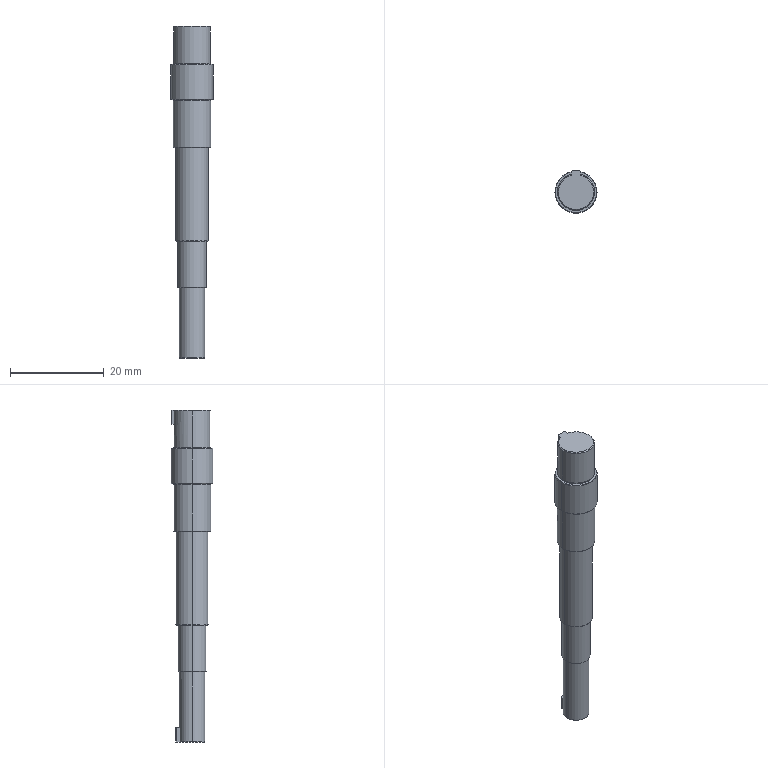Part | SolidWorks | features ICE 9, Chamfer 2, Fillet 2, Extrusion 1 | 1 solid | 53 faces | box 9 x 9 x 71 mm | volume 2813 mm3 | cylinder 20 | plane 17 | cone 16 | commonest cylinder face diameters 0.4 x4 7.8 x4 5.5 x2 6 x2 7 x2 7.9 x2
STEP:
#1=CARTESIAN_POINT('',(-2.65,0.,-63.));
#2=VERTEX_POINT('',#1);
#3=CARTESIAN_POINT('',(-1.,2.454,-63.));
#4=VERTEX_POINT('',#3);
#5=CARTESIAN_POINT('',(0.,0.,-63.));
#6=DIRECTION('',(0.,0.,-1.));
#7=DIRECTION('',(-1.,0.,0.));
#8=AXIS2_PLACEMENT_3D('',#5,#6,#7);
#9=CIRCLE('',#8,2.65);
#10=EDGE_CURVE('',#2,#4,#9,.T.);
#11=ORIENTED_EDGE('',*,*,#10,.F.);
#12=CARTESIAN_POINT('',(-2.75,0.,-62.9));
#13=VERTEX_POINT('',#12);
#14=CARTESIAN_POINT('',(-2.65,0.,-63.));
#15=DIRECTION('',(-0.7071,0.,0.7071));
#16=VECTOR('',#15,1000.);
#17=LINE('',#14,#16);
#18=EDGE_CURVE('',#2,#13,#17,.T.);
#19=ORIENTED_EDGE('',*,*,#18,.T.);
#20=CARTESIAN_POINT('',(-1.,2.562,-62.9));
#21=VERTEX_POINT('',#20);
#22=CARTESIAN_POINT('',(0.,0.,-62.9));
#23=DIRECTION('',(0.,0.,1.));
#24=DIRECTION('',(-1.,0.,0.));
#25=AXIS2_PLACEMENT_3D('',#22,#23,#24);
#26=CIRCLE('',#25,2.75);
#27=EDGE_CURVE('',#21,#13,#26,.T.);
#28=ORIENTED_EDGE('',*,*,#27,.F.);
#29=CARTESIAN_POINT('',(-1.,2.454,-63.));
#30=CARTESIAN_POINT('',(-1.,2.49,-62.967));
#31=CARTESIAN_POINT('',(-1.,2.526,-62.933));
#32=CARTESIAN_POINT('',(-1.,2.562,-62.9));
#33=B_SPLINE_CURVE_WITH_KNOTS('',3,(#29,#30,#31,#32),.UNSPECIFIED.,.F.,.F.,(4,4),(0.,0.0001469),.UNSPECIFIED.);
#34=EDGE_CURVE('',#4,#21,#33,.T.);
#35=ORIENTED_EDGE('',*,*,#34,.F.);
#36=EDGE_LOOP('',(#11,#19,#28,#35));
#37=FACE_OUTER_BOUND('',#36,.T.);
#38=CARTESIAN_POINT('',(0.,0.,-63.));
#39=DIRECTION('',(0.,0.,1.));
#40=DIRECTION('',(1.,0.,0.));
#41=AXIS2_PLACEMENT_3D('',#38,#39,#40);
#42=CONICAL_SURFACE('',#41,2.65,0.7854);
#43=ADVANCED_FACE('',(#37),#42,.T.);
#44=ORIENTED_EDGE('',*,*,#18,.F.);
#45=CARTESIAN_POINT('',(2.65,0.,-63.));
#46=VERTEX_POINT('',#45);
#47=CARTESIAN_POINT('',(0.,0.,-63.));
#48=DIRECTION('',(0.,0.,-1.));
#49=DIRECTION('',(-1.,0.,0.));
#50=AXIS2_PLACEMENT_3D('',#47,#48,#49);
#51=CIRCLE('',#50,2.65);
#52=EDGE_CURVE('',#46,#2,#51,.T.);
#53=ORIENTED_EDGE('',*,*,#52,.F.);
#54=CARTESIAN_POINT('',(2.75,0.,-62.9));
#55=VERTEX_POINT('',#54);
#56=CARTESIAN_POINT('',(2.65,0.,-63.));
#57=DIRECTION('',(0.7071,0.,0.7071));
#58=VECTOR('',#57,1000.);
#59=LINE('',#56,#58);
#60=EDGE_CURVE('',#46,#55,#59,.T.);
#61=ORIENTED_EDGE('',*,*,#60,.T.);
#62=CARTESIAN_POINT('',(0.,0.,-62.9));
#63=DIRECTION('',(0.,0.,1.));
#64=DIRECTION('',(-1.,0.,0.));
#65=AXIS2_PLACEMENT_3D('',#62,#63,#64);
#66=CIRCLE('',#65,2.75);
#67=EDGE_CURVE('',#13,#55,#66,.T.);
#68=ORIENTED_EDGE('',*,*,#67,.F.);
#69=EDGE_LOOP('',(#44,#53,#61,#68));
#70=FACE_OUTER_BOUND('',#69,.T.);
#71=CARTESIAN_POINT('',(0.,0.,-63.));
#72=DIRECTION('',(0.,0.,1.));
#73=DIRECTION('',(1.,0.,0.));
#74=AXIS2_PLACEMENT_3D('',#71,#72,#73);
#75=CONICAL_SURFACE('',#74,2.65,0.7854);
#76=ADVANCED_FACE('',(#70),#75,.T.);
#77=CARTESIAN_POINT('',(-2.9,0.,-48.));
#78=VERTEX_POINT('',#77);
#79=CARTESIAN_POINT('',(2.9,0.,-48.));
#80=VERTEX_POINT('',#79);
#81=CARTESIAN_POINT('',(0.,0.,-48.));
#82=DIRECTION('',(0.,0.,-1.));
#83=DIRECTION('',(-1.,0.,0.));
#84=AXIS2_PLACEMENT_3D('',#81,#82,#83);
#85=CIRCLE('',#84,2.9);
#86=EDGE_CURVE('',#78,#80,#85,.T.);
#87=ORIENTED_EDGE('',*,*,#86,.F.);
#88=CARTESIAN_POINT('',(-3.,0.,-47.9));
#89=VERTEX_POINT('',#88);
#90=CARTESIAN_POINT('',(-2.9,0.,-48.));
#91=DIRECTION('',(-0.7071,0.,0.7071));
#92=VECTOR('',#91,1000.);
#93=LINE('',#90,#92);
#94=EDGE_CURVE('',#78,#89,#93,.T.);
#95=ORIENTED_EDGE('',*,*,#94,.T.);
#96=CARTESIAN_POINT('',(3.,0.,-47.9));
#97=VERTEX_POINT('',#96);
#98=CARTESIAN_POINT('',(0.,0.,-47.9));
#99=DIRECTION('',(0.,0.,1.));
#100=DIRECTION('',(-1.,0.,0.));
#101=AXIS2_PLACEMENT_3D('',#98,#99,#100);
#102=CIRCLE('',#101,3.);
#103=EDGE_CURVE('',#97,#89,#102,.T.);
#104=ORIENTED_EDGE('',*,*,#103,.F.);
#105=CARTESIAN_POINT('',(2.9,0.,-48.));
#106=DIRECTION('',(0.7071,0.,0.7071));
#107=VECTOR('',#106,1000.);
#108=LINE('',#105,#107);
#109=EDGE_CURVE('',#80,#97,#108,.T.);
#110=ORIENTED_EDGE('',*,*,#109,.F.);
#111=EDGE_LOOP('',(#87,#95,#104,#110));
#112=FACE_OUTER_BOUND('',#111,.T.);
#113=CARTESIAN_POINT('',(0.,0.,-48.));
#114=DIRECTION('',(0.,0.,1.));
#115=DIRECTION('',(1.,0.,0.));
#116=AXIS2_PLACEMENT_3D('',#113,#114,#115);
#117=CONICAL_SURFACE('',#116,2.9,0.7854);
#118=ADVANCED_FACE('',(#112),#117,.T.);
#119=CARTESIAN_POINT('',(-3.4,0.,-38.));
#120=VERTEX_POINT('',#119);
#121=CARTESIAN_POINT('',(3.4,0.,-38.));
#122=VERTEX_POINT('',#121);
#123=CARTESIAN_POINT('',(0.,0.,-38.));
#124=DIRECTION('',(0.,0.,-1.));
#125=DIRECTION('',(-1.,0.,0.));
#126=AXIS2_PLACEMENT_3D('',#123,#124,#125);
#127=CIRCLE('',#126,3.4);
#128=EDGE_CURVE('',#120,#122,#127,.T.);
#129=ORIENTED_EDGE('',*,*,#128,.F.);
#130=CARTESIAN_POINT('',(-3.5,0.,-37.9));
#131=VERTEX_POINT('',#130);
#132=CARTESIAN_POINT('',(-3.4,0.,-38.));
#133=DIRECTION('',(-0.7071,0.,0.7071));
#134=VECTOR('',#133,1000.);
#135=LINE('',#132,#134);
#136=EDGE_CURVE('',#120,#131,#135,.T.);
#137=ORIENTED_EDGE('',*,*,#136,.T.);
#138=CARTESIAN_POINT('',(3.5,0.,-37.9));
#139=VERTEX_POINT('',#138);
#140=CARTESIAN_POINT('',(0.,0.,-37.9));
#141=DIRECTION('',(0.,0.,1.));
#142=DIRECTION('',(-1.,0.,0.));
#143=AXIS2_PLACEMENT_3D('',#140,#141,#142);
#144=CIRCLE('',#143,3.5);
#145=EDGE_CURVE('',#139,#131,#144,.T.);
#146=ORIENTED_EDGE('',*,*,#145,.F.);
#147=CARTESIAN_POINT('',(3.4,0.,-38.));
#148=DIRECTION('',(0.7071,0.,0.7071));
#149=VECTOR('',#148,1000.);
#150=LINE('',#147,#149);
#151=EDGE_CURVE('',#122,#139,#150,.T.);
#152=ORIENTED_EDGE('',*,*,#151,.F.);
#153=EDGE_LOOP('',(#129,#137,#146,#152));
#154=FACE_OUTER_BOUND('',#153,.T.);
#155=CARTESIAN_POINT('',(0.,0.,-38.));
#156=DIRECTION('',(0.,0.,1.));
#157=DIRECTION('',(1.,0.,0.));
#158=AXIS2_PLACEMENT_3D('',#155,#156,#157);
#159=CONICAL_SURFACE('',#158,3.4,0.7854);
#160=ADVANCED_FACE('',(#154),#159,.T.);
#161=CARTESIAN_POINT('',(-3.9,0.,-18.));
#162=VERTEX_POINT('',#161);
#163=CARTESIAN_POINT('',(3.9,0.,-18.));
#164=VERTEX_POINT('',#163);
#165=CARTESIAN_POINT('',(0.,0.,-18.));
#166=DIRECTION('',(0.,0.,-1.));
#167=DIRECTION('',(-1.,0.,0.));
#168=AXIS2_PLACEMENT_3D('',#165,#166,#167);
#169=CIRCLE('',#168,3.9);
#170=EDGE_CURVE('',#162,#164,#169,.T.);
#171=ORIENTED_EDGE('',*,*,#170,.F.);
#172=CARTESIAN_POINT('',(-4.,0.,-17.9));
#173=VERTEX_POINT('',#172);
#174=CARTESIAN_POINT('',(-3.9,0.,-18.));
#175=DIRECTION('',(-0.7071,0.,0.7071));
#176=VECTOR('',#175,1000.);
#177=LINE('',#174,#176);
#178=EDGE_CURVE('',#162,#173,#177,.T.);
#179=ORIENTED_EDGE('',*,*,#178,.T.);
#180=CARTESIAN_POINT('',(4.,0.,-17.9));
#181=VERTEX_POINT('',#180);
#182=CARTESIAN_POINT('',(0.,0.,-17.9));
#183=DIRECTION('',(0.,0.,1.));
#184=DIRECTION('',(-1.,0.,0.));
#185=AXIS2_PLACEMENT_3D('',#182,#183,#184);
#186=CIRCLE('',#185,4.);
#187=EDGE_CURVE('',#181,#173,#186,.T.);
#188=ORIENTED_EDGE('',*,*,#187,.F.);
#189=CARTESIAN_POINT('',(3.9,0.,-18.));
#190=DIRECTION('',(0.7071,0.,0.7071));
#191=VECTOR('',#190,1000.);
#192=LINE('',#189,#191);
#193=EDGE_CURVE('',#164,#181,#192,.T.);
#194=ORIENTED_EDGE('',*,*,#193,.F.);
#195=EDGE_LOOP('',(#171,#179,#188,#194));
#196=FACE_OUTER_BOUND('',#195,.T.);
#197=CARTESIAN_POINT('',(0.,0.,-18.));
#198=DIRECTION('',(0.,0.,1.));
#199=DIRECTION('',(1.,0.,0.));
#200=AXIS2_PLACEMENT_3D('',#197,#198,#199);
#201=CONICAL_SURFACE('',#200,3.9,0.7854);
#202=ADVANCED_FACE('',(#196),#201,.T.);
#203=CARTESIAN_POINT('',(-4.4,0.,-7.8));
#204=VERTEX_POINT('',#203);
#205=CARTESIAN_POINT('',(4.4,0.,-7.8));
#206=VERTEX_POINT('',#205);
#207=CARTESIAN_POINT('',(0.,0.,-7.8));
#208=DIRECTION('',(0.,0.,-1.));
#209=DIRECTION('',(-1.,0.,0.));
#210=AXIS2_PLACEMENT_3D('',#207,#208,#209);
#211=CIRCLE('',#210,4.4);
#212=EDGE_CURVE('',#204,#206,#211,.T.);
#213=ORIENTED_EDGE('',*,*,#212,.F.);
#214=CARTESIAN_POINT('',(-4.5,0.,-7.7));
#215=VERTEX_POINT('',#214);
#216=CARTESIAN_POINT('',(-4.4,0.,-7.8));
#217=DIRECTION('',(-0.7071,0.,0.7071));
#218=VECTOR('',#217,1000.);
#219=LINE('',#216,#218);
#220=EDGE_CURVE('',#204,#215,#219,.T.);
#221=ORIENTED_EDGE('',*,*,#220,.T.);
#222=CARTESIAN_POINT('',(4.5,0.,-7.7));
#223=VERTEX_POINT('',#222);
#224=CARTESIAN_POINT('',(0.,0.,-7.7));
#225=DIRECTION('',(0.,0.,1.));
#226=DIRECTION('',(-1.,0.,0.));
#227=AXIS2_PLACEMENT_3D('',#224,#225,#226);
#228=CIRCLE('',#227,4.5);
#229=EDGE_CURVE('',#223,#215,#228,.T.);
#230=ORIENTED_EDGE('',*,*,#229,.F.);
#231=CARTESIAN_POINT('',(4.4,0.,-7.8));
#232=DIRECTION('',(0.7071,0.,0.7071));
#233=VECTOR('',#232,1000.);
#234=LINE('',#231,#233);
#235=EDGE_CURVE('',#206,#223,#234,.T.);
#236=ORIENTED_EDGE('',*,*,#235,.F.);
#237=EDGE_LOOP('',(#213,#221,#230,#236));
#238=FACE_OUTER_BOUND('',#237,.T.);
#239=CARTESIAN_POINT('',(0.,0.,-7.8));
#240=DIRECTION('',(0.,0.,1.));
#241=DIRECTION('',(1.,0.,0.));
#242=AXIS2_PLACEMENT_3D('',#239,#240,#241);
#243=CONICAL_SURFACE('',#242,4.4,0.7854);
#244=ADVANCED_FACE('',(#238),#243,.T.);
#245=CARTESIAN_POINT('',(4.4,0.,-0.2));
#246=VERTEX_POINT('',#245);
#247=CARTESIAN_POINT('',(-4.4,0.,-0.2));
#248=VERTEX_POINT('',#247);
#249=CARTESIAN_POINT('',(0.,0.,-0.2));
#250=DIRECTION('',(0.,0.,1.));
#251=DIRECTION('',(-1.,0.,0.));
#252=AXIS2_PLACEMENT_3D('',#249,#250,#251);
#253=CIRCLE('',#252,4.4);
#254=EDGE_CURVE('',#246,#248,#253,.T.);
#255=ORIENTED_EDGE('',*,*,#254,.F.);
#256=CARTESIAN_POINT('',(4.5,0.,-0.3));
#257=VERTEX_POINT('',#256);
#258=CARTESIAN_POINT('',(4.5,0.,-0.3));
#259=DIRECTION('',(0.7071,0.,-0.7071));
#260=VECTOR('',#259,1000.);
#261=LINE('',#258,#260);
#262=EDGE_CURVE('',#246,#257,#261,.T.);
#263=ORIENTED_EDGE('',*,*,#262,.T.);
#264=CARTESIAN_POINT('',(-4.5,0.,-0.3));
#265=VERTEX_POINT('',#264);
#266=CARTESIAN_POINT('',(0.,0.,-0.3));
#267=DIRECTION('',(0.,0.,-1.));
#268=DIRECTION('',(-1.,0.,0.));
#269=AXIS2_PLACEMENT_3D('',#266,#267,#268);
#270=CIRCLE('',#269,4.5);
#271=EDGE_CURVE('',#265,#257,#270,.T.);
#272=ORIENTED_EDGE('',*,*,#271,.F.);
#273=CARTESIAN_POINT('',(-4.5,0.,-0.3));
#274=DIRECTION('',(-0.7071,0.,-0.7071));
#275=VECTOR('',#274,1000.);
#276=LINE('',#273,#275);
#277=EDGE_CURVE('',#248,#265,#276,.T.);
#278=ORIENTED_EDGE('',*,*,#277,.F.);
#279=EDGE_LOOP('',(#255,#263,#272,#278));
#280=FACE_OUTER_BOUND('',#279,.T.);
#281=CARTESIAN_POINT('',(0.,0.,-0.3));
#282=DIRECTION('',(0.,0.,-1.));
#283=DIRECTION('',(-1.,0.,0.));
#284=AXIS2_PLACEMENT_3D('',#281,#282,#283);
#285=CONICAL_SURFACE('',#284,4.5,0.7854);
#286=ADVANCED_FACE('',(#280),#285,.T.);
#287=ORIENTED_EDGE('',*,*,#27,.T.);
#288=CARTESIAN_POINT('',(-2.75,0.,-48.));
#289=VERTEX_POINT('',#288);
#290=CARTESIAN_POINT('',(-2.75,0.,-63.));
#291=DIRECTION('',(0.,0.,1.));
#292=VECTOR('',#291,1000.);
#293=LINE('',#290,#292);
#294=EDGE_CURVE('',#13,#289,#293,.T.);
#295=ORIENTED_EDGE('',*,*,#294,.T.);
#296=CARTESIAN_POINT('',(2.75,0.,-48.));
#297=VERTEX_POINT('',#296);
#298=CARTESIAN_POINT('',(0.,0.,-48.));
#299=DIRECTION('',(0.,0.,-1.));
#300=DIRECTION('',(-1.,0.,0.));
#301=AXIS2_PLACEMENT_3D('',#298,#299,#300);
#302=CIRCLE('',#301,2.75);
#303=EDGE_CURVE('',#289,#297,#302,.T.);
#304=ORIENTED_EDGE('',*,*,#303,.T.);
#305=CARTESIAN_POINT('',(2.75,0.,-63.));
#306=DIRECTION('',(0.,0.,1.));
#307=VECTOR('',#306,1000.);
#308=LINE('',#305,#307);
#309=EDGE_CURVE('',#55,#297,#308,.T.);
#310=ORIENTED_EDGE('',*,*,#309,.F.);
#311=CARTESIAN_POINT('',(1.,2.562,-62.9));
#312=VERTEX_POINT('',#311);
#313=CARTESIAN_POINT('',(0.,0.,-62.9));
#314=DIRECTION('',(0.,0.,1.));
#315=DIRECTION('',(-1.,0.,0.));
#316=AXIS2_PLACEMENT_3D('',#313,#314,#315);
#317=CIRCLE('',#316,2.75);
#318=EDGE_CURVE('',#55,#312,#317,.T.);
#319=ORIENTED_EDGE('',*,*,#318,.T.);
#320=CARTESIAN_POINT('',(1.,2.562,-60.));
#321=VERTEX_POINT('',#320);
#322=CARTESIAN_POINT('',(1.,2.562,-65.209));
#323=DIRECTION('',(0.,0.,1.));
#324=VECTOR('',#323,1000.);
#325=LINE('',#322,#324);
#326=EDGE_CURVE('',#312,#321,#325,.T.);
#327=ORIENTED_EDGE('',*,*,#326,.T.);
#328=CARTESIAN_POINT('',(-1.,2.562,-60.));
#329=VERTEX_POINT('',#328);
#330=CARTESIAN_POINT('',(0.,0.,-60.));
#331=DIRECTION('',(0.,0.,-1.));
#332=DIRECTION('',(-1.,0.,0.));
#333=AXIS2_PLACEMENT_3D('',#330,#331,#332);
#334=CIRCLE('',#333,2.75);
#335=EDGE_CURVE('',#329,#321,#334,.T.);
#336=ORIENTED_EDGE('',*,*,#335,.F.);
#337=CARTESIAN_POINT('',(-1.,2.562,-65.209));
#338=DIRECTION('',(0.,0.,1.));
#339=VECTOR('',#338,1000.);
#340=LINE('',#337,#339);
#341=EDGE_CURVE('',#21,#329,#340,.T.);
#342=ORIENTED_EDGE('',*,*,#341,.F.);
#343=EDGE_LOOP('',(#287,#295,#304,#310,#319,#327,#336,#342));
#344=FACE_OUTER_BOUND('',#343,.T.);
#345=CARTESIAN_POINT('',(0.,0.,-63.));
#346=DIRECTION('',(0.,0.,1.));
#347=DIRECTION('',(1.,0.,0.));
#348=AXIS2_PLACEMENT_3D('',#345,#346,#347);
#349=CYLINDRICAL_SURFACE('',#348,2.75);
#350=ADVANCED_FACE('',(#344),#349,.T.);
#351=ORIENTED_EDGE('',*,*,#103,.T.);
#352=CARTESIAN_POINT('',(-3.,0.,-38.));
#353=VERTEX_POINT('',#352);
#354=CARTESIAN_POINT('',(-3.,0.,-48.));
#355=DIRECTION('',(0.,0.,1.));
#356=VECTOR('',#355,1000.);
#357=LINE('',#354,#356);
#358=EDGE_CURVE('',#89,#353,#357,.T.);
#359=ORIENTED_EDGE('',*,*,#358,.T.);
#360=CARTESIAN_POINT('',(3.,0.,-38.));
#361=VERTEX_POINT('',#360);
#362=CARTESIAN_POINT('',(0.,0.,-38.));
#363=DIRECTION('',(0.,0.,-1.));
#364=DIRECTION('',(-1.,0.,0.));
#365=AXIS2_PLACEMENT_3D('',#362,#363,#364);
#366=CIRCLE('',#365,3.);
#367=EDGE_CURVE('',#353,#361,#366,.T.);
#368=ORIENTED_EDGE('',*,*,#367,.T.);
#369=CARTESIAN_POINT('',(3.,0.,-48.));
#370=DIRECTION('',(0.,0.,1.));
#371=VECTOR('',#370,1000.);
#372=LINE('',#369,#371);
#373=EDGE_CURVE('',#97,#361,#372,.T.);
#374=ORIENTED_EDGE('',*,*,#373,.F.);
#375=EDGE_LOOP('',(#351,#359,#368,#374));
#376=FACE_OUTER_BOUND('',#375,.T.);
#377=CARTESIAN_POINT('',(0.,0.,-48.));
#378=DIRECTION('',(0.,0.,1.));
#379=DIRECTION('',(1.,0.,0.));
#380=AXIS2_PLACEMENT_3D('',#377,#378,#379);
#381=CYLINDRICAL_SURFACE('',#380,3.);
#382=ADVANCED_FACE('',(#376),#381,.T.);
#383=ORIENTED_EDGE('',*,*,#145,.T.);
#384=CARTESIAN_POINT('',(-3.5,0.,-18.));
#385=VERTEX_POINT('',#384);
#386=CARTESIAN_POINT('',(-3.5,0.,-38.));
#387=DIRECTION('',(0.,0.,1.));
#388=VECTOR('',#387,1000.);
#389=LINE('',#386,#388);
#390=EDGE_CURVE('',#131,#385,#389,.T.);
#391=ORIENTED_EDGE('',*,*,#390,.T.);
#392=CARTESIAN_POINT('',(3.5,0.,-18.));
#393=VERTEX_POINT('',#392);
#394=CARTESIAN_POINT('',(0.,0.,-18.));
#395=DIRECTION('',(0.,0.,-1.));
#396=DIRECTION('',(-1.,0.,0.));
#397=AXIS2_PLACEMENT_3D('',#394,#395,#396);
#398=CIRCLE('',#397,3.5);
#399=EDGE_CURVE('',#385,#393,#398,.T.);
#400=ORIENTED_EDGE('',*,*,#399,.T.);
#401=CARTESIAN_POINT('',(3.5,0.,-38.));
#402=DIRECTION('',(0.,0.,1.));
#403=VECTOR('',#402,1000.);
#404=LINE('',#401,#403);
#405=EDGE_CURVE('',#139,#393,#404,.T.);
#406=ORIENTED_EDGE('',*,*,#405,.F.);
#407=EDGE_LOOP('',(#383,#391,#400,#406));
#408=FACE_OUTER_BOUND('',#407,.T.);
#409=CARTESIAN_POINT('',(0.,0.,-38.));
#410=DIRECTION('',(0.,0.,1.));
#411=DIRECTION('',(1.,0.,0.));
#412=AXIS2_PLACEMENT_3D('',#409,#410,#411);
#413=CYLINDRICAL_SURFACE('',#412,3.5);
#414=ADVANCED_FACE('',(#408),#413,.T.);
#415=ORIENTED_EDGE('',*,*,#187,.T.);
#416=CARTESIAN_POINT('',(-4.,0.,-8.));
#417=VERTEX_POINT('',#416);
#418=CARTESIAN_POINT('',(-4.,0.,-18.));
#419=DIRECTION('',(0.,0.,1.));
#420=VECTOR('',#419,1000.);
#421=LINE('',#418,#420);
#422=EDGE_CURVE('',#173,#417,#421,.T.);
#423=ORIENTED_EDGE('',*,*,#422,.T.);
#424=CARTESIAN_POINT('',(4.,0.,-8.));
#425=VERTEX_POINT('',#424);
#426=CARTESIAN_POINT('',(0.,0.,-8.));
#427=DIRECTION('',(0.,0.,-1.));
#428=DIRECTION('',(-1.,0.,0.));
#429=AXIS2_PLACEMENT_3D('',#426,#427,#428);
#430=CIRCLE('',#429,4.);
#431=EDGE_CURVE('',#417,#425,#430,.T.);
#432=ORIENTED_EDGE('',*,*,#431,.T.);
#433=CARTESIAN_POINT('',(4.,0.,-18.));
#434=DIRECTION('',(0.,0.,1.));
#435=VECTOR('',#434,1000.);
#436=LINE('',#433,#435);
#437=EDGE_CURVE('',#181,#425,#436,.T.);
#438=ORIENTED_EDGE('',*,*,#437,.F.);
#439=EDGE_LOOP('',(#415,#423,#432,#438));
#440=FACE_OUTER_BOUND('',#439,.T.);
#441=CARTESIAN_POINT('',(0.,0.,-18.));
#442=DIRECTION('',(0.,0.,1.));
#443=DIRECTION('',(1.,0.,0.));
#444=AXIS2_PLACEMENT_3D('',#441,#442,#443);
#445=CYLINDRICAL_SURFACE('',#444,4.);
#446=ADVANCED_FACE('',(#440),#445,.T.);
#447=CARTESIAN_POINT('',(3.75,0.,8.));
#448=VERTEX_POINT('',#447);
#449=CARTESIAN_POINT('',(1.,3.614,8.));
#450=VERTEX_POINT('',#449);
#451=CARTESIAN_POINT('',(0.,0.,8.));
#452=DIRECTION('',(0.,0.,1.));
#453=DIRECTION('',(1.,0.,0.));
#454=AXIS2_PLACEMENT_3D('',#451,#452,#453);
#455=CIRCLE('',#454,3.75);
#456=EDGE_CURVE('',#448,#450,#455,.T.);
#457=ORIENTED_EDGE('',*,*,#456,.F.);
#458=CARTESIAN_POINT('',(3.95,0.,7.8));
#459=VERTEX_POINT('',#458);
#460=CARTESIAN_POINT('',(3.75,0.,8.));
#461=DIRECTION('',(0.7071,0.,-0.7071));
#462=VECTOR('',#461,1000.);
#463=LINE('',#460,#462);
#464=EDGE_CURVE('',#448,#459,#463,.T.);
#465=ORIENTED_EDGE('',*,*,#464,.T.);
#466=CARTESIAN_POINT('',(1.,3.821,7.8));
#467=VERTEX_POINT('',#466);
#468=CARTESIAN_POINT('',(0.,0.,7.8));
#469=DIRECTION('',(0.,0.,-1.));
#470=DIRECTION('',(1.,0.,0.));
#471=AXIS2_PLACEMENT_3D('',#468,#469,#470);
#472=CIRCLE('',#471,3.95);
#473=EDGE_CURVE('',#467,#459,#472,.T.);
#474=ORIENTED_EDGE('',*,*,#473,.F.);
#475=CARTESIAN_POINT('',(1.,3.614,8.));
#476=CARTESIAN_POINT('',(1.,3.683,7.933));
#477=CARTESIAN_POINT('',(1.,3.752,7.867));
#478=CARTESIAN_POINT('',(1.,3.821,7.8));
#479=B_SPLINE_CURVE_WITH_KNOTS('',3,(#475,#476,#477,#478),.UNSPECIFIED.,.F.,.F.,(4,4),(0.,0.0002879),.UNSPECIFIED.);
#480=EDGE_CURVE('',#450,#467,#479,.T.);
#481=ORIENTED_EDGE('',*,*,#480,.F.);
#482=EDGE_LOOP('',(#457,#465,#474,#481));
#483=FACE_OUTER_BOUND('',#482,.T.);
#484=CARTESIAN_POINT('',(0.,0.,8.));
#485=DIRECTION('',(0.,0.,-1.));
#486=DIRECTION('',(-1.,0.,0.));
#487=AXIS2_PLACEMENT_3D('',#484,#485,#486);
#488=CONICAL_SURFACE('',#487,3.75,0.7854);
#489=ADVANCED_FACE('',(#483),#488,.T.);
#490=ORIENTED_EDGE('',*,*,#464,.F.);
#491=CARTESIAN_POINT('',(-3.75,0.,8.));
#492=VERTEX_POINT('',#491);
#493=CARTESIAN_POINT('',(0.,0.,8.));
#494=DIRECTION('',(0.,0.,1.));
#495=DIRECTION('',(1.,0.,0.));
#496=AXIS2_PLACEMENT_3D('',#493,#494,#495);
#497=CIRCLE('',#496,3.75);
#498=EDGE_CURVE('',#492,#448,#497,.T.);
#499=ORIENTED_EDGE('',*,*,#498,.F.);
#500=CARTESIAN_POINT('',(-3.95,0.,7.8));
#501=VERTEX_POINT('',#500);
#502=CARTESIAN_POINT('',(-3.75,0.,8.));
#503=DIRECTION('',(-0.7071,0.,-0.7071));
#504=VECTOR('',#503,1000.);
#505=LINE('',#502,#504);
#506=EDGE_CURVE('',#492,#501,#505,.T.);
#507=ORIENTED_EDGE('',*,*,#506,.T.);
#508=CARTESIAN_POINT('',(0.,0.,7.8));
#509=DIRECTION('',(0.,0.,-1.));
#510=DIRECTION('',(1.,0.,0.));
#511=AXIS2_PLACEMENT_3D('',#508,#509,#510);
#512=CIRCLE('',#511,3.95);
#513=EDGE_CURVE('',#459,#501,#512,.T.);
#514=ORIENTED_EDGE('',*,*,#513,.F.);
#515=EDGE_LOOP('',(#490,#499,#507,#514));
#516=FACE_OUTER_BOUND('',#515,.T.);
#517=CARTESIAN_POINT('',(0.,0.,8.));
#518=DIRECTION('',(0.,0.,-1.));
#519=DIRECTION('',(-1.,0.,0.));
#520=AXIS2_PLACEMENT_3D('',#517,#518,#519);
#521=CONICAL_SURFACE('',#520,3.75,0.7854);
#522=ADVANCED_FACE('',(#516),#521,.T.);
#523=CARTESIAN_POINT('',(-3.9,0.,-8.));
#524=VERTEX_POINT('',#523);
#525=CARTESIAN_POINT('',(3.9,0.,-8.));
#526=VERTEX_POINT('',#525);
#527=CARTESIAN_POINT('',(0.,0.,-8.));
#528=DIRECTION('',(0.,0.,-1.));
#529=DIRECTION('',(-1.,0.,0.));
#530=AXIS2_PLACEMENT_3D('',#527,#528,#529);
#531=CIRCLE('',#530,3.9);
#532=EDGE_CURVE('',#524,#526,#531,.T.);
#533=ORIENTED_EDGE('',*,*,#532,.F.);
#534=CARTESIAN_POINT('',(-3.9,0.,-7.8));
#535=VERTEX_POINT('',#534);
#536=CARTESIAN_POINT('',(-3.9,0.,-8.));
#537=DIRECTION('',(0.,0.,1.));
#538=VECTOR('',#537,1000.);
#539=LINE('',#536,#538);
#540=EDGE_CURVE('',#524,#535,#539,.T.);
#541=ORIENTED_EDGE('',*,*,#540,.T.);
#542=CARTESIAN_POINT('',(3.9,0.,-7.8));
#543=VERTEX_POINT('',#542);
#544=CARTESIAN_POINT('',(0.,0.,-7.8));
#545=DIRECTION('',(0.,0.,-1.));
#546=DIRECTION('',(-1.,0.,0.));
#547=AXIS2_PLACEMENT_3D('',#544,#545,#546);
#548=CIRCLE('',#547,3.9);
#549=EDGE_CURVE('',#535,#543,#548,.T.);
#550=ORIENTED_EDGE('',*,*,#549,.T.);
#551=CARTESIAN_POINT('',(3.9,0.,-8.));
#552=DIRECTION('',(0.,0.,1.));
#553=VECTOR('',#552,1000.);
#554=LINE('',#551,#553);
#555=EDGE_CURVE('',#526,#543,#554,.T.);
#556=ORIENTED_EDGE('',*,*,#555,.F.);
#557=EDGE_LOOP('',(#533,#541,#550,#556));
#558=FACE_OUTER_BOUND('',#557,.T.);
#559=CARTESIAN_POINT('',(0.,0.,-8.));
#560=DIRECTION('',(0.,0.,1.));
#561=DIRECTION('',(1.,0.,0.));
#562=AXIS2_PLACEMENT_3D('',#559,#560,#561);
#563=CYLINDRICAL_SURFACE('',#562,3.9);
#564=ADVANCED_FACE('',(#558),#563,.T.);
#565=ORIENTED_EDGE('',*,*,#229,.T.);
#566=CARTESIAN_POINT('',(-4.5,0.,-7.8));
#567=DIRECTION('',(0.,0.,1.));
#568=VECTOR('',#567,1000.);
#569=LINE('',#566,#568);
#570=EDGE_CURVE('',#215,#265,#569,.T.);
#571=ORIENTED_EDGE('',*,*,#570,.T.);
#572=ORIENTED_EDGE('',*,*,#271,.T.);
#573=CARTESIAN_POINT('',(4.5,0.,-7.8));
#574=DIRECTION('',(0.,0.,1.));
#575=VECTOR('',#574,1000.);
#576=LINE('',#573,#575);
#577=EDGE_CURVE('',#223,#257,#576,.T.);
#578=ORIENTED_EDGE('',*,*,#577,.F.);
#579=EDGE_LOOP('',(#565,#571,#572,#578));
#580=FACE_OUTER_BOUND('',#579,.T.);
#581=CARTESIAN_POINT('',(0.,0.,-7.8));
#582=DIRECTION('',(0.,0.,1.));
#583=DIRECTION('',(1.,0.,0.));
#584=AXIS2_PLACEMENT_3D('',#581,#582,#583);
#585=CYLINDRICAL_SURFACE('',#584,4.5);
#586=ADVANCED_FACE('',(#580),#585,.T.);
#587=CARTESIAN_POINT('',(-3.9,0.,-0.2));
#588=VERTEX_POINT('',#587);
#589=CARTESIAN_POINT('',(3.9,0.,-0.2));
#590=VERTEX_POINT('',#589);
#591=CARTESIAN_POINT('',(0.,0.,-0.2));
#592=DIRECTION('',(0.,0.,-1.));
#593=DIRECTION('',(-1.,0.,0.));
#594=AXIS2_PLACEMENT_3D('',#591,#592,#593);
#595=CIRCLE('',#594,3.9);
#596=EDGE_CURVE('',#588,#590,#595,.T.);
#597=ORIENTED_EDGE('',*,*,#596,.F.);
#598=CARTESIAN_POINT('',(-3.9,0.,0.));
#599=VERTEX_POINT('',#598);
#600=CARTESIAN_POINT('',(-3.9,0.,-0.2));
#601=DIRECTION('',(0.,0.,1.));
#602=VECTOR('',#601,1000.);
#603=LINE('',#600,#602);
#604=EDGE_CURVE('',#588,#599,#603,.T.);
#605=ORIENTED_EDGE('',*,*,#604,.T.);
#606=CARTESIAN_POINT('',(3.9,0.,0.));
#607=VERTEX_POINT('',#606);
#608=CARTESIAN_POINT('',(0.,0.,0.));
#609=DIRECTION('',(0.,0.,-1.));
#610=DIRECTION('',(-1.,0.,0.));
#611=AXIS2_PLACEMENT_3D('',#608,#609,#610);
#612=CIRCLE('',#611,3.9);
#613=EDGE_CURVE('',#599,#607,#612,.T.);
#614=ORIENTED_EDGE('',*,*,#613,.T.);
#615=CARTESIAN_POINT('',(3.9,0.,-0.2));
#616=DIRECTION('',(0.,0.,1.));
#617=VECTOR('',#616,1000.);
#618=LINE('',#615,#617);
#619=EDGE_CURVE('',#590,#607,#618,.T.);
#620=ORIENTED_EDGE('',*,*,#619,.F.);
#621=EDGE_LOOP('',(#597,#605,#614,#620));
#622=FACE_OUTER_BOUND('',#621,.T.);
#623=CARTESIAN_POINT('',(0.,0.,-0.2));
#624=DIRECTION('',(0.,0.,1.));
#625=DIRECTION('',(1.,0.,0.));
#626=AXIS2_PLACEMENT_3D('',#623,#624,#625);
#627=CYLINDRICAL_SURFACE('',#626,3.9);
#628=ADVANCED_FACE('',(#622),#627,.T.);
#629=ORIENTED_EDGE('',*,*,#473,.T.);
#630=CARTESIAN_POINT('',(3.95,0.,0.));
#631=VERTEX_POINT('',#630);
#632=CARTESIAN_POINT('',(3.95,0.,8.));
#633=DIRECTION('',(0.,0.,-1.));
#634=VECTOR('',#633,1000.);
#635=LINE('',#632,#634);
#636=EDGE_CURVE('',#459,#631,#635,.T.);
#637=ORIENTED_EDGE('',*,*,#636,.T.);
#638=CARTESIAN_POINT('',(-3.95,0.,0.));
#639=VERTEX_POINT('',#638);
#640=CARTESIAN_POINT('',(0.,0.,0.));
#641=DIRECTION('',(0.,0.,1.));
#642=DIRECTION('',(1.,0.,0.));
#643=AXIS2_PLACEMENT_3D('',#640,#641,#642);
#644=CIRCLE('',#643,3.95);
#645=EDGE_CURVE('',#631,#639,#644,.T.);
#646=ORIENTED_EDGE('',*,*,#645,.T.);
#647=CARTESIAN_POINT('',(-3.95,0.,8.));
#648=DIRECTION('',(0.,0.,-1.));
#649=VECTOR('',#648,1000.);
#650=LINE('',#647,#649);
#651=EDGE_CURVE('',#501,#639,#650,.T.);
#652=ORIENTED_EDGE('',*,*,#651,.F.);
#653=CARTESIAN_POINT('',(-1.,3.821,7.8));
#654=VERTEX_POINT('',#653);
#655=CARTESIAN_POINT('',(0.,0.,7.8));
#656=DIRECTION('',(0.,0.,-1.));
#657=DIRECTION('',(1.,0.,0.));
#658=AXIS2_PLACEMENT_3D('',#655,#656,#657);
#659=CIRCLE('',#658,3.95);
#660=EDGE_CURVE('',#501,#654,#659,.T.);
#661=ORIENTED_EDGE('',*,*,#660,.T.);
#662=CARTESIAN_POINT('',(-1.,3.821,5.));
#663=VERTEX_POINT('',#662);
#664=CARTESIAN_POINT('',(-1.,3.821,8.));
#665=DIRECTION('',(0.,0.,-1.));
#666=VECTOR('',#665,1000.);
#667=LINE('',#664,#666);
#668=EDGE_CURVE('',#654,#663,#667,.T.);
#669=ORIENTED_EDGE('',*,*,#668,.T.);
#670=CARTESIAN_POINT('',(1.,3.821,5.));
#671=VERTEX_POINT('',#670);
#672=CARTESIAN_POINT('',(0.,0.,5.));
#673=DIRECTION('',(0.,0.,-1.));
#674=DIRECTION('',(-1.,0.,0.));
#675=AXIS2_PLACEMENT_3D('',#672,#673,#674);
#676=CIRCLE('',#675,3.95);
#677=EDGE_CURVE('',#663,#671,#676,.T.);
#678=ORIENTED_EDGE('',*,*,#677,.T.);
#679=CARTESIAN_POINT('',(1.,3.821,8.));
#680=DIRECTION('',(0.,0.,1.));
#681=VECTOR('',#680,1000.);
#682=LINE('',#679,#681);
#683=EDGE_CURVE('',#671,#467,#682,.T.);
#684=ORIENTED_EDGE('',*,*,#683,.T.);
#685=EDGE_LOOP('',(#629,#637,#646,#652,#661,#669,#678,#684));
#686=FACE_OUTER_BOUND('',#685,.T.);
#687=CARTESIAN_POINT('',(0.,0.,8.));
#688=DIRECTION('',(0.,0.,-1.));
#689=DIRECTION('',(-1.,0.,0.));
#690=AXIS2_PLACEMENT_3D('',#687,#688,#689);
#691=CYLINDRICAL_SURFACE('',#690,3.95);
#692=ADVANCED_FACE('',(#686),#691,.T.);
#693=ORIENTED_EDGE('',*,*,#636,.F.);
#694=ORIENTED_EDGE('',*,*,#513,.T.);
#695=ORIENTED_EDGE('',*,*,#651,.T.);
#696=CARTESIAN_POINT('',(0.,0.,0.));
#697=DIRECTION('',(0.,0.,1.));
#698=DIRECTION('',(1.,0.,0.));
#699=AXIS2_PLACEMENT_3D('',#696,#697,#698);
#700=CIRCLE('',#699,3.95);
#701=EDGE_CURVE('',#639,#631,#700,.T.);
#702=ORIENTED_EDGE('',*,*,#701,.T.);
#703=EDGE_LOOP('',(#693,#694,#695,#702));
#704=FACE_OUTER_BOUND('',#703,.T.);
#705=CARTESIAN_POINT('',(0.,0.,8.));
#706=DIRECTION('',(0.,0.,-1.));
#707=DIRECTION('',(-1.,0.,0.));
#708=AXIS2_PLACEMENT_3D('',#705,#706,#707);
#709=CYLINDRICAL_SURFACE('',#708,3.95);
#710=ADVANCED_FACE('',(#704),#709,.T.);
#711=CARTESIAN_POINT('',(-1.,3.614,8.));
#712=VERTEX_POINT('',#711);
#713=CARTESIAN_POINT('',(0.,0.,8.));
#714=DIRECTION('',(0.,0.,1.));
#715=DIRECTION('',(1.,0.,0.));
#716=AXIS2_PLACEMENT_3D('',#713,#714,#715);
#717=CIRCLE('',#716,3.75);
#718=EDGE_CURVE('',#712,#492,#717,.T.);
#719=ORIENTED_EDGE('',*,*,#718,.T.);
#720=ORIENTED_EDGE('',*,*,#498,.T.);
#721=ORIENTED_EDGE('',*,*,#456,.T.);
#722=CARTESIAN_POINT('',(1.,4.3,8.));
#723=VERTEX_POINT('',#722);
#724=CARTESIAN_POINT('',(1.,4.5,8.));
#725=DIRECTION('',(0.,-1.,0.));
#726=VECTOR('',#725,1000.);
#727=LINE('',#724,#726);
#728=EDGE_CURVE('',#723,#450,#727,.T.);
#729=ORIENTED_EDGE('',*,*,#728,.F.);
#730=CARTESIAN_POINT('',(0.8,4.5,8.));
#731=VERTEX_POINT('',#730);
#732=CARTESIAN_POINT('',(0.8,4.3,8.));
#733=DIRECTION('',(0.,0.,1.));
#734=DIRECTION('',(1.,0.,0.));
#735=AXIS2_PLACEMENT_3D('',#732,#733,#734);
#736=CIRCLE('',#735,0.2);
#737=EDGE_CURVE('',#723,#731,#736,.T.);
#738=ORIENTED_EDGE('',*,*,#737,.T.);
#739=CARTESIAN_POINT('',(-0.8,4.5,8.));
#740=VERTEX_POINT('',#739);
#741=CARTESIAN_POINT('',(1.,4.5,8.));
#742=DIRECTION('',(1.,0.,0.));
#743=VECTOR('',#742,1000.);
#744=LINE('',#741,#743);
#745=EDGE_CURVE('',#740,#731,#744,.T.);
#746=ORIENTED_EDGE('',*,*,#745,.F.);
#747=CARTESIAN_POINT('',(-1.,4.3,8.));
#748=VERTEX_POINT('',#747);
#749=CARTESIAN_POINT('',(-0.8,4.3,8.));
#750=DIRECTION('',(0.,0.,1.));
#751=DIRECTION('',(1.,0.,0.));
#752=AXIS2_PLACEMENT_3D('',#749,#750,#751);
#753=CIRCLE('',#752,0.2);
#754=EDGE_CURVE('',#740,#748,#753,.T.);
#755=ORIENTED_EDGE('',*,*,#754,.T.);
#756=CARTESIAN_POINT('',(-1.,4.5,8.));
#757=DIRECTION('',(0.,1.,0.));
#758=VECTOR('',#757,1000.);
#759=LINE('',#756,#758);
#760=EDGE_CURVE('',#712,#748,#759,.T.);
#761=ORIENTED_EDGE('',*,*,#760,.F.);
#762=EDGE_LOOP('',(#719,#720,#721,#729,#738,#746,#755,#761));
#763=FACE_OUTER_BOUND('',#762,.T.);
#764=CARTESIAN_POINT('',(0.,0.,8.));
#765=DIRECTION('',(0.,0.,1.));
#766=DIRECTION('',(1.,0.,0.));
#767=AXIS2_PLACEMENT_3D('',#764,#765,#766);
#768=PLANE('',#767);
#769=ADVANCED_FACE('',(#763),#768,.T.);
#770=CARTESIAN_POINT('',(0.,0.,0.));
#771=DIRECTION('',(0.,0.,-1.));
#772=DIRECTION('',(-1.,0.,0.));
#773=AXIS2_PLACEMENT_3D('',#770,#771,#772);
#774=CIRCLE('',#773,3.9);
#775=EDGE_CURVE('',#607,#599,#774,.T.);
#776=ORIENTED_EDGE('',*,*,#775,.F.);
#777=ORIENTED_EDGE('',*,*,#613,.F.);
#778=EDGE_LOOP('',(#776,#777));
#779=FACE_BOUND('',#778,.T.);
#780=ORIENTED_EDGE('',*,*,#701,.F.);
#781=ORIENTED_EDGE('',*,*,#645,.F.);
#782=EDGE_LOOP('',(#780,#781));
#783=FACE_OUTER_BOUND('',#782,.T.);
#784=CARTESIAN_POINT('',(0.,0.,0.));
#785=DIRECTION('',(0.,0.,1.));
#786=DIRECTION('',(1.,0.,0.));
#787=AXIS2_PLACEMENT_3D('',#784,#785,#786);
#788=PLANE('',#787);
#789=ADVANCED_FACE('',(#779,#783),#788,.F.);
#790=ORIENTED_EDGE('',*,*,#760,.T.);
#791=CARTESIAN_POINT('',(-1.,4.3,5.));
#792=VERTEX_POINT('',#791);
#793=CARTESIAN_POINT('',(-1.,4.3,10.5));
#794=DIRECTION('',(0.,0.,-1.));
#795=VECTOR('',#794,1000.);
#796=LINE('',#793,#795);
#797=EDGE_CURVE('',#748,#792,#796,.T.);
#798=ORIENTED_EDGE('',*,*,#797,.T.);
#799=CARTESIAN_POINT('',(-1.,4.5,5.));
#800=DIRECTION('',(0.,1.,0.));
#801=VECTOR('',#800,1000.);
#802=LINE('',#799,#801);
#803=EDGE_CURVE('',#663,#792,#802,.T.);
#804=ORIENTED_EDGE('',*,*,#803,.F.);
#805=ORIENTED_EDGE('',*,*,#668,.F.);
#806=CARTESIAN_POINT('',(-1.,3.821,7.8));
#807=CARTESIAN_POINT('',(-1.,3.752,7.867));
#808=CARTESIAN_POINT('',(-1.,3.683,7.933));
#809=CARTESIAN_POINT('',(-1.,3.614,8.));
#810=B_SPLINE_CURVE_WITH_KNOTS('',3,(#806,#807,#808,#809),.UNSPECIFIED.,.F.,.F.,(4,4),(0.,0.0002879),.UNSPECIFIED.);
#811=EDGE_CURVE('',#654,#712,#810,.T.);
#812=ORIENTED_EDGE('',*,*,#811,.T.);
#813=EDGE_LOOP('',(#790,#798,#804,#805,#812));
#814=FACE_OUTER_BOUND('',#813,.T.);
#815=CARTESIAN_POINT('',(-1.,4.5,10.5));
#816=DIRECTION('',(-1.,0.,0.));
#817=DIRECTION('',(0.,0.,1.));
#818=AXIS2_PLACEMENT_3D('',#815,#816,#817);
#819=PLANE('',#818);
#820=ADVANCED_FACE('',(#814),#819,.T.);
#821=CARTESIAN_POINT('',(1.,4.3,5.));
#822=VERTEX_POINT('',#821);
#823=CARTESIAN_POINT('',(1.,4.5,5.));
#824=DIRECTION('',(0.,-1.,0.));
#825=VECTOR('',#824,1000.);
#826=LINE('',#823,#825);
#827=EDGE_CURVE('',#822,#671,#826,.T.);
#828=ORIENTED_EDGE('',*,*,#827,.F.);
#829=CARTESIAN_POINT('',(1.,4.3,10.5));
#830=DIRECTION('',(0.,0.,1.));
#831=VECTOR('',#830,1000.);
#832=LINE('',#829,#831);
#833=EDGE_CURVE('',#822,#723,#832,.T.);
#834=ORIENTED_EDGE('',*,*,#833,.T.);
#835=ORIENTED_EDGE('',*,*,#728,.T.);
#836=ORIENTED_EDGE('',*,*,#480,.T.);
#837=ORIENTED_EDGE('',*,*,#683,.F.);
#838=EDGE_LOOP('',(#828,#834,#835,#836,#837));
#839=FACE_OUTER_BOUND('',#838,.T.);
#840=CARTESIAN_POINT('',(1.,4.5,10.5));
#841=DIRECTION('',(1.,0.,0.));
#842=DIRECTION('',(0.,0.,-1.));
#843=AXIS2_PLACEMENT_3D('',#840,#841,#842);
#844=PLANE('',#843);
#845=ADVANCED_FACE('',(#839),#844,.T.);
#846=CARTESIAN_POINT('',(-0.8,4.5,5.));
#847=VERTEX_POINT('',#846);
#848=CARTESIAN_POINT('',(0.8,4.5,5.));
#849=VERTEX_POINT('',#848);
#850=CARTESIAN_POINT('',(1.,4.5,5.));
#851=DIRECTION('',(1.,0.,0.));
#852=VECTOR('',#851,1000.);
#853=LINE('',#850,#852);
#854=EDGE_CURVE('',#847,#849,#853,.T.);
#855=ORIENTED_EDGE('',*,*,#854,.T.);
#856=CARTESIAN_POINT('',(0.8,4.3,5.));
#857=DIRECTION('',(0.,0.,-1.));
#858=DIRECTION('',(-1.,0.,0.));
#859=AXIS2_PLACEMENT_3D('',#856,#857,#858);
#860=CIRCLE('',#859,0.2);
#861=EDGE_CURVE('',#849,#822,#860,.T.);
#862=ORIENTED_EDGE('',*,*,#861,.T.);
#863=ORIENTED_EDGE('',*,*,#827,.T.);
#864=ORIENTED_EDGE('',*,*,#677,.F.);
#865=ORIENTED_EDGE('',*,*,#803,.T.);
#866=CARTESIAN_POINT('',(-0.8,4.3,5.));
#867=DIRECTION('',(0.,0.,-1.));
#868=DIRECTION('',(-1.,0.,0.));
#869=AXIS2_PLACEMENT_3D('',#866,#867,#868);
#870=CIRCLE('',#869,0.2);
#871=EDGE_CURVE('',#792,#847,#870,.T.);
#872=ORIENTED_EDGE('',*,*,#871,.T.);
#873=EDGE_LOOP('',(#855,#862,#863,#864,#865,#872));
#874=FACE_OUTER_BOUND('',#873,.T.);
#875=CARTESIAN_POINT('',(0.,0.,5.));
#876=DIRECTION('',(0.,0.,-1.));
#877=DIRECTION('',(-1.,0.,0.));
#878=AXIS2_PLACEMENT_3D('',#875,#876,#877);
#879=PLANE('',#878);
#880=ADVANCED_FACE('',(#874),#879,.T.);
#881=ORIENTED_EDGE('',*,*,#745,.T.);
#882=CARTESIAN_POINT('',(0.8,4.5,10.5));
#883=DIRECTION('',(0.,0.,-1.));
#884=VECTOR('',#883,1000.);
#885=LINE('',#882,#884);
#886=EDGE_CURVE('',#731,#849,#885,.T.);
#887=ORIENTED_EDGE('',*,*,#886,.T.);
#888=ORIENTED_EDGE('',*,*,#854,.F.);
#889=CARTESIAN_POINT('',(-0.8,4.5,10.5));
#890=DIRECTION('',(0.,0.,1.));
#891=VECTOR('',#890,1000.);
#892=LINE('',#889,#891);
#893=EDGE_CURVE('',#847,#740,#892,.T.);
#894=ORIENTED_EDGE('',*,*,#893,.T.);
#895=EDGE_LOOP('',(#881,#887,#888,#894));
#896=FACE_OUTER_BOUND('',#895,.T.);
#897=CARTESIAN_POINT('',(1.,4.5,10.5));
#898=DIRECTION('',(0.,1.,0.));
#899=DIRECTION('',(0.,0.,1.));
#900=AXIS2_PLACEMENT_3D('',#897,#898,#899);
#901=PLANE('',#900);
#902=ADVANCED_FACE('',(#896),#901,.T.);
#903=ORIENTED_EDGE('',*,*,#737,.F.);
#904=ORIENTED_EDGE('',*,*,#833,.F.);
#905=ORIENTED_EDGE('',*,*,#861,.F.);
#906=ORIENTED_EDGE('',*,*,#886,.F.);
#907=EDGE_LOOP('',(#903,#904,#905,#906));
#908=FACE_OUTER_BOUND('',#907,.T.);
#909=CARTESIAN_POINT('',(0.8,4.3,10.5));
#910=DIRECTION('',(0.,0.,-1.));
#911=DIRECTION('',(-1.,0.,0.));
#912=AXIS2_PLACEMENT_3D('',#909,#910,#911);
#913=CYLINDRICAL_SURFACE('',#912,0.2);
#914=ADVANCED_FACE('',(#908),#913,.T.);
#915=ORIENTED_EDGE('',*,*,#754,.F.);
#916=ORIENTED_EDGE('',*,*,#893,.F.);
#917=ORIENTED_EDGE('',*,*,#871,.F.);
#918=ORIENTED_EDGE('',*,*,#797,.F.);
#919=EDGE_LOOP('',(#915,#916,#917,#918));
#920=FACE_OUTER_BOUND('',#919,.T.);
#921=CARTESIAN_POINT('',(-0.8,4.3,10.5));
#922=DIRECTION('',(0.,0.,-1.));
#923=DIRECTION('',(-1.,0.,0.));
#924=AXIS2_PLACEMENT_3D('',#921,#922,#923);
#925=CYLINDRICAL_SURFACE('',#924,0.2);
#926=ADVANCED_FACE('',(#920),#925,.T.);
#927=ORIENTED_EDGE('',*,*,#604,.F.);
#928=CARTESIAN_POINT('',(0.,0.,-0.2));
#929=DIRECTION('',(0.,0.,-1.));
#930=DIRECTION('',(-1.,0.,0.));
#931=AXIS2_PLACEMENT_3D('',#928,#929,#930);
#932=CIRCLE('',#931,3.9);
#933=EDGE_CURVE('',#590,#588,#932,.T.);
#934=ORIENTED_EDGE('',*,*,#933,.F.);
#935=ORIENTED_EDGE('',*,*,#619,.T.);
#936=ORIENTED_EDGE('',*,*,#775,.T.);
#937=EDGE_LOOP('',(#927,#934,#935,#936));
#938=FACE_OUTER_BOUND('',#937,.T.);
#939=CARTESIAN_POINT('',(0.,0.,-0.2));
#940=DIRECTION('',(0.,0.,1.));
#941=DIRECTION('',(1.,0.,0.));
#942=AXIS2_PLACEMENT_3D('',#939,#940,#941);
#943=CYLINDRICAL_SURFACE('',#942,3.9);
#944=ADVANCED_FACE('',(#938),#943,.T.);
#945=ORIENTED_EDGE('',*,*,#570,.F.);
#946=CARTESIAN_POINT('',(0.,0.,-7.7));
#947=DIRECTION('',(0.,0.,1.));
#948=DIRECTION('',(-1.,0.,0.));
#949=AXIS2_PLACEMENT_3D('',#946,#947,#948);
#950=CIRCLE('',#949,4.5);
#951=EDGE_CURVE('',#215,#223,#950,.T.);
#952=ORIENTED_EDGE('',*,*,#951,.T.);
#953=ORIENTED_EDGE('',*,*,#577,.T.);
#954=CARTESIAN_POINT('',(0.,0.,-0.3));
#955=DIRECTION('',(0.,0.,-1.));
#956=DIRECTION('',(-1.,0.,0.));
#957=AXIS2_PLACEMENT_3D('',#954,#955,#956);
#958=CIRCLE('',#957,4.5);
#959=EDGE_CURVE('',#257,#265,#958,.T.);
#960=ORIENTED_EDGE('',*,*,#959,.T.);
#961=EDGE_LOOP('',(#945,#952,#953,#960));
#962=FACE_OUTER_BOUND('',#961,.T.);
#963=CARTESIAN_POINT('',(0.,0.,-7.8));
#964=DIRECTION('',(0.,0.,1.));
#965=DIRECTION('',(1.,0.,0.));
#966=AXIS2_PLACEMENT_3D('',#963,#964,#965);
#967=CYLINDRICAL_SURFACE('',#966,4.5);
#968=ADVANCED_FACE('',(#962),#967,.T.);
#969=CARTESIAN_POINT('',(0.,0.,-7.8));
#970=DIRECTION('',(0.,0.,-1.));
#971=DIRECTION('',(-1.,0.,0.));
#972=AXIS2_PLACEMENT_3D('',#969,#970,#971);
#973=CIRCLE('',#972,4.4);
#974=EDGE_CURVE('',#206,#204,#973,.T.);
#975=ORIENTED_EDGE('',*,*,#974,.T.);
#976=ORIENTED_EDGE('',*,*,#212,.T.);
#977=EDGE_LOOP('',(#975,#976));
#978=FACE_OUTER_BOUND('',#977,.T.);
#979=CARTESIAN_POINT('',(0.,0.,-7.8));
#980=DIRECTION('',(0.,0.,-1.));
#981=DIRECTION('',(-1.,0.,0.));
#982=AXIS2_PLACEMENT_3D('',#979,#980,#981);
#983=CIRCLE('',#982,3.9);
#984=EDGE_CURVE('',#543,#535,#983,.T.);
#985=ORIENTED_EDGE('',*,*,#984,.F.);
#986=ORIENTED_EDGE('',*,*,#549,.F.);
#987=EDGE_LOOP('',(#985,#986));
#988=FACE_BOUND('',#987,.T.);
#989=CARTESIAN_POINT('',(0.,0.,-7.8));
#990=DIRECTION('',(0.,0.,-1.));
#991=DIRECTION('',(-1.,0.,0.));
#992=AXIS2_PLACEMENT_3D('',#989,#990,#991);
#993=PLANE('',#992);
#994=ADVANCED_FACE('',(#978,#988),#993,.T.);
#995=CARTESIAN_POINT('',(0.,0.,-0.2));
#996=DIRECTION('',(0.,0.,1.));
#997=DIRECTION('',(-1.,0.,0.));
#998=AXIS2_PLACEMENT_3D('',#995,#996,#997);
#999=CIRCLE('',#998,4.4);
#1000=EDGE_CURVE('',#248,#246,#999,.T.);
#1001=ORIENTED_EDGE('',*,*,#1000,.T.);
#1002=ORIENTED_EDGE('',*,*,#254,.T.);
#1003=EDGE_LOOP('',(#1001,#1002));
#1004=FACE_OUTER_BOUND('',#1003,.T.);
#1005=ORIENTED_EDGE('',*,*,#933,.T.);
#1006=ORIENTED_EDGE('',*,*,#596,.T.);
#1007=EDGE_LOOP('',(#1005,#1006));
#1008=FACE_BOUND('',#1007,.T.);
#1009=CARTESIAN_POINT('',(0.,0.,-0.2));
#1010=DIRECTION('',(0.,0.,-1.));
#1011=DIRECTION('',(-1.,0.,0.));
#1012=AXIS2_PLACEMENT_3D('',#1009,#1010,#1011);
#1013=PLANE('',#1012);
#1014=ADVANCED_FACE('',(#1004,#1008),#1013,.F.);
#1015=ORIENTED_EDGE('',*,*,#540,.F.);
#1016=CARTESIAN_POINT('',(0.,0.,-8.));
#1017=DIRECTION('',(0.,0.,-1.));
#1018=DIRECTION('',(-1.,0.,0.));
#1019=AXIS2_PLACEMENT_3D('',#1016,#1017,#1018);
#1020=CIRCLE('',#1019,3.9);
#1021=EDGE_CURVE('',#526,#524,#1020,.T.);
#1022=ORIENTED_EDGE('',*,*,#1021,.F.);
#1023=ORIENTED_EDGE('',*,*,#555,.T.);
#1024=ORIENTED_EDGE('',*,*,#984,.T.);
#1025=EDGE_LOOP('',(#1015,#1022,#1023,#1024));
#1026=FACE_OUTER_BOUND('',#1025,.T.);
#1027=CARTESIAN_POINT('',(0.,0.,-8.));
#1028=DIRECTION('',(0.,0.,1.));
#1029=DIRECTION('',(1.,0.,0.));
#1030=AXIS2_PLACEMENT_3D('',#1027,#1028,#1029);
#1031=CYLINDRICAL_SURFACE('',#1030,3.9);
#1032=ADVANCED_FACE('',(#1026),#1031,.T.);
#1033=ORIENTED_EDGE('',*,*,#506,.F.);
#1034=ORIENTED_EDGE('',*,*,#718,.F.);
#1035=ORIENTED_EDGE('',*,*,#811,.F.);
#1036=ORIENTED_EDGE('',*,*,#660,.F.);
#1037=EDGE_LOOP('',(#1033,#1034,#1035,#1036));
#1038=FACE_OUTER_BOUND('',#1037,.T.);
#1039=CARTESIAN_POINT('',(0.,0.,8.));
#1040=DIRECTION('',(0.,0.,-1.));
#1041=DIRECTION('',(-1.,0.,0.));
#1042=AXIS2_PLACEMENT_3D('',#1039,#1040,#1041);
#1043=CONICAL_SURFACE('',#1042,3.75,0.7854);
#1044=ADVANCED_FACE('',(#1038),#1043,.T.);
#1045=ORIENTED_EDGE('',*,*,#422,.F.);
#1046=CARTESIAN_POINT('',(0.,0.,-17.9));
#1047=DIRECTION('',(0.,0.,1.));
#1048=DIRECTION('',(-1.,0.,0.));
#1049=AXIS2_PLACEMENT_3D('',#1046,#1047,#1048);
#1050=CIRCLE('',#1049,4.);
#1051=EDGE_CURVE('',#173,#181,#1050,.T.);
#1052=ORIENTED_EDGE('',*,*,#1051,.T.);
#1053=ORIENTED_EDGE('',*,*,#437,.T.);
#1054=CARTESIAN_POINT('',(0.,0.,-8.));
#1055=DIRECTION('',(0.,0.,-1.));
#1056=DIRECTION('',(-1.,0.,0.));
#1057=AXIS2_PLACEMENT_3D('',#1054,#1055,#1056);
#1058=CIRCLE('',#1057,4.);
#1059=EDGE_CURVE('',#425,#417,#1058,.T.);
#1060=ORIENTED_EDGE('',*,*,#1059,.T.);
#1061=EDGE_LOOP('',(#1045,#1052,#1053,#1060));
#1062=FACE_OUTER_BOUND('',#1061,.T.);
#1063=CARTESIAN_POINT('',(0.,0.,-18.));
#1064=DIRECTION('',(0.,0.,1.));
#1065=DIRECTION('',(1.,0.,0.));
#1066=AXIS2_PLACEMENT_3D('',#1063,#1064,#1065);
#1067=CYLINDRICAL_SURFACE('',#1066,4.);
#1068=ADVANCED_FACE('',(#1062),#1067,.T.);
#1069=CARTESIAN_POINT('',(0.,0.,-18.));
#1070=DIRECTION('',(0.,0.,-1.));
#1071=DIRECTION('',(-1.,0.,0.));
#1072=AXIS2_PLACEMENT_3D('',#1069,#1070,#1071);
#1073=CIRCLE('',#1072,3.9);
#1074=EDGE_CURVE('',#164,#162,#1073,.T.);
#1075=ORIENTED_EDGE('',*,*,#1074,.T.);
#1076=ORIENTED_EDGE('',*,*,#170,.T.);
#1077=EDGE_LOOP('',(#1075,#1076));
#1078=FACE_OUTER_BOUND('',#1077,.T.);
#1079=CARTESIAN_POINT('',(0.,0.,-18.));
#1080=DIRECTION('',(0.,0.,-1.));
#1081=DIRECTION('',(-1.,0.,0.));
#1082=AXIS2_PLACEMENT_3D('',#1079,#1080,#1081);
#1083=CIRCLE('',#1082,3.5);
#1084=EDGE_CURVE('',#393,#385,#1083,.T.);
#1085=ORIENTED_EDGE('',*,*,#1084,.F.);
#1086=ORIENTED_EDGE('',*,*,#399,.F.);
#1087=EDGE_LOOP('',(#1085,#1086));
#1088=FACE_BOUND('',#1087,.T.);
#1089=CARTESIAN_POINT('',(0.,0.,-18.));
#1090=DIRECTION('',(0.,0.,-1.));
#1091=DIRECTION('',(-1.,0.,0.));
#1092=AXIS2_PLACEMENT_3D('',#1089,#1090,#1091);
#1093=PLANE('',#1092);
#1094=ADVANCED_FACE('',(#1078,#1088),#1093,.T.);
#1095=ORIENTED_EDGE('',*,*,#1021,.T.);
#1096=ORIENTED_EDGE('',*,*,#532,.T.);
#1097=EDGE_LOOP('',(#1095,#1096));
#1098=FACE_BOUND('',#1097,.T.);
#1099=ORIENTED_EDGE('',*,*,#1059,.F.);
#1100=ORIENTED_EDGE('',*,*,#431,.F.);
#1101=EDGE_LOOP('',(#1099,#1100));
#1102=FACE_OUTER_BOUND('',#1101,.T.);
#1103=CARTESIAN_POINT('',(0.,0.,-8.));
#1104=DIRECTION('',(0.,0.,-1.));
#1105=DIRECTION('',(-1.,0.,0.));
#1106=AXIS2_PLACEMENT_3D('',#1103,#1104,#1105);
#1107=PLANE('',#1106);
#1108=ADVANCED_FACE('',(#1098,#1102),#1107,.F.);
#1109=ORIENTED_EDGE('',*,*,#390,.F.);
#1110=CARTESIAN_POINT('',(0.,0.,-37.9));
#1111=DIRECTION('',(0.,0.,1.));
#1112=DIRECTION('',(-1.,0.,0.));
#1113=AXIS2_PLACEMENT_3D('',#1110,#1111,#1112);
#1114=CIRCLE('',#1113,3.5);
#1115=EDGE_CURVE('',#131,#139,#1114,.T.);
#1116=ORIENTED_EDGE('',*,*,#1115,.T.);
#1117=ORIENTED_EDGE('',*,*,#405,.T.);
#1118=ORIENTED_EDGE('',*,*,#1084,.T.);
#1119=EDGE_LOOP('',(#1109,#1116,#1117,#1118));
#1120=FACE_OUTER_BOUND('',#1119,.T.);
#1121=CARTESIAN_POINT('',(0.,0.,-38.));
#1122=DIRECTION('',(0.,0.,1.));
#1123=DIRECTION('',(1.,0.,0.));
#1124=AXIS2_PLACEMENT_3D('',#1121,#1122,#1123);
#1125=CYLINDRICAL_SURFACE('',#1124,3.5);
#1126=ADVANCED_FACE('',(#1120),#1125,.T.);
#1127=CARTESIAN_POINT('',(0.,0.,-38.));
#1128=DIRECTION('',(0.,0.,-1.));
#1129=DIRECTION('',(-1.,0.,0.));
#1130=AXIS2_PLACEMENT_3D('',#1127,#1128,#1129);
#1131=CIRCLE('',#1130,3.4);
#1132=EDGE_CURVE('',#122,#120,#1131,.T.);
#1133=ORIENTED_EDGE('',*,*,#1132,.T.);
#1134=ORIENTED_EDGE('',*,*,#128,.T.);
#1135=EDGE_LOOP('',(#1133,#1134));
#1136=FACE_OUTER_BOUND('',#1135,.T.);
#1137=CARTESIAN_POINT('',(0.,0.,-38.));
#1138=DIRECTION('',(0.,0.,-1.));
#1139=DIRECTION('',(-1.,0.,0.));
#1140=AXIS2_PLACEMENT_3D('',#1137,#1138,#1139);
#1141=CIRCLE('',#1140,3.);
#1142=EDGE_CURVE('',#361,#353,#1141,.T.);
#1143=ORIENTED_EDGE('',*,*,#1142,.F.);
#1144=ORIENTED_EDGE('',*,*,#367,.F.);
#1145=EDGE_LOOP('',(#1143,#1144));
#1146=FACE_BOUND('',#1145,.T.);
#1147=CARTESIAN_POINT('',(0.,0.,-38.));
#1148=DIRECTION('',(0.,0.,-1.));
#1149=DIRECTION('',(-1.,0.,0.));
#1150=AXIS2_PLACEMENT_3D('',#1147,#1148,#1149);
#1151=PLANE('',#1150);
#1152=ADVANCED_FACE('',(#1136,#1146),#1151,.T.);
#1153=ORIENTED_EDGE('',*,*,#358,.F.);
#1154=CARTESIAN_POINT('',(0.,0.,-47.9));
#1155=DIRECTION('',(0.,0.,1.));
#1156=DIRECTION('',(-1.,0.,0.));
#1157=AXIS2_PLACEMENT_3D('',#1154,#1155,#1156);
#1158=CIRCLE('',#1157,3.);
#1159=EDGE_CURVE('',#89,#97,#1158,.T.);
#1160=ORIENTED_EDGE('',*,*,#1159,.T.);
#1161=ORIENTED_EDGE('',*,*,#373,.T.);
#1162=ORIENTED_EDGE('',*,*,#1142,.T.);
#1163=EDGE_LOOP('',(#1153,#1160,#1161,#1162));
#1164=FACE_OUTER_BOUND('',#1163,.T.);
#1165=CARTESIAN_POINT('',(0.,0.,-48.));
#1166=DIRECTION('',(0.,0.,1.));
#1167=DIRECTION('',(1.,0.,0.));
#1168=AXIS2_PLACEMENT_3D('',#1165,#1166,#1167);
#1169=CYLINDRICAL_SURFACE('',#1168,3.);
#1170=ADVANCED_FACE('',(#1164),#1169,.T.);
#1171=CARTESIAN_POINT('',(0.,0.,-48.));
#1172=DIRECTION('',(0.,0.,-1.));
#1173=DIRECTION('',(-1.,0.,0.));
#1174=AXIS2_PLACEMENT_3D('',#1171,#1172,#1173);
#1175=CIRCLE('',#1174,2.9);
#1176=EDGE_CURVE('',#80,#78,#1175,.T.);
#1177=ORIENTED_EDGE('',*,*,#1176,.T.);
#1178=ORIENTED_EDGE('',*,*,#86,.T.);
#1179=EDGE_LOOP('',(#1177,#1178));
#1180=FACE_OUTER_BOUND('',#1179,.T.);
#1181=CARTESIAN_POINT('',(0.,0.,-48.));
#1182=DIRECTION('',(0.,0.,-1.));
#1183=DIRECTION('',(-1.,0.,0.));
#1184=AXIS2_PLACEMENT_3D('',#1181,#1182,#1183);
#1185=CIRCLE('',#1184,2.75);
#1186=EDGE_CURVE('',#297,#289,#1185,.T.);
#1187=ORIENTED_EDGE('',*,*,#1186,.F.);
#1188=ORIENTED_EDGE('',*,*,#303,.F.);
#1189=EDGE_LOOP('',(#1187,#1188));
#1190=FACE_BOUND('',#1189,.T.);
#1191=CARTESIAN_POINT('',(0.,0.,-48.));
#1192=DIRECTION('',(0.,0.,-1.));
#1193=DIRECTION('',(-1.,0.,0.));
#1194=AXIS2_PLACEMENT_3D('',#1191,#1192,#1193);
#1195=PLANE('',#1194);
#1196=ADVANCED_FACE('',(#1180,#1190),#1195,.T.);
#1197=ORIENTED_EDGE('',*,*,#294,.F.);
#1198=ORIENTED_EDGE('',*,*,#67,.T.);
#1199=ORIENTED_EDGE('',*,*,#309,.T.);
#1200=ORIENTED_EDGE('',*,*,#1186,.T.);
#1201=EDGE_LOOP('',(#1197,#1198,#1199,#1200));
#1202=FACE_OUTER_BOUND('',#1201,.T.);
#1203=CARTESIAN_POINT('',(0.,0.,-63.));
#1204=DIRECTION('',(0.,0.,1.));
#1205=DIRECTION('',(1.,0.,0.));
#1206=AXIS2_PLACEMENT_3D('',#1203,#1204,#1205);
#1207=CYLINDRICAL_SURFACE('',#1206,2.75);
#1208=ADVANCED_FACE('',(#1202),#1207,.T.);
#1209=CARTESIAN_POINT('',(1.,2.454,-63.));
#1210=VERTEX_POINT('',#1209);
#1211=CARTESIAN_POINT('',(0.,0.,-63.));
#1212=DIRECTION('',(0.,0.,-1.));
#1213=DIRECTION('',(-1.,0.,0.));
#1214=AXIS2_PLACEMENT_3D('',#1211,#1212,#1213);
#1215=CIRCLE('',#1214,2.65);
#1216=EDGE_CURVE('',#1210,#46,#1215,.T.);
#1217=ORIENTED_EDGE('',*,*,#1216,.T.);
#1218=ORIENTED_EDGE('',*,*,#52,.T.);
#1219=ORIENTED_EDGE('',*,*,#10,.T.);
#1220=CARTESIAN_POINT('',(-1.,3.3,-63.));
#1221=VERTEX_POINT('',#1220);
#1222=CARTESIAN_POINT('',(-1.,3.5,-63.));
#1223=DIRECTION('',(0.,-1.,0.));
#1224=VECTOR('',#1223,1000.);
#1225=LINE('',#1222,#1224);
#1226=EDGE_CURVE('',#1221,#4,#1225,.T.);
#1227=ORIENTED_EDGE('',*,*,#1226,.F.);
#1228=CARTESIAN_POINT('',(-0.8,3.5,-63.));
#1229=VERTEX_POINT('',#1228);
#1230=CARTESIAN_POINT('',(-0.8,3.3,-63.));
#1231=DIRECTION('',(0.,0.,-1.));
#1232=DIRECTION('',(-1.,0.,0.));
#1233=AXIS2_PLACEMENT_3D('',#1230,#1231,#1232);
#1234=CIRCLE('',#1233,0.2);
#1235=EDGE_CURVE('',#1221,#1229,#1234,.T.);
#1236=ORIENTED_EDGE('',*,*,#1235,.T.);
#1237=CARTESIAN_POINT('',(0.8,3.5,-63.));
#1238=VERTEX_POINT('',#1237);
#1239=CARTESIAN_POINT('',(1.,3.5,-63.));
#1240=DIRECTION('',(-1.,0.,0.));
#1241=VECTOR('',#1240,1000.);
#1242=LINE('',#1239,#1241);
#1243=EDGE_CURVE('',#1238,#1229,#1242,.T.);
#1244=ORIENTED_EDGE('',*,*,#1243,.F.);
#1245=CARTESIAN_POINT('',(1.,3.3,-63.));
#1246=VERTEX_POINT('',#1245);
#1247=CARTESIAN_POINT('',(0.8,3.3,-63.));
#1248=DIRECTION('',(0.,0.,-1.));
#1249=DIRECTION('',(-1.,0.,0.));
#1250=AXIS2_PLACEMENT_3D('',#1247,#1248,#1249);
#1251=CIRCLE('',#1250,0.2);
#1252=EDGE_CURVE('',#1238,#1246,#1251,.T.);
#1253=ORIENTED_EDGE('',*,*,#1252,.T.);
#1254=CARTESIAN_POINT('',(1.,3.5,-63.));
#1255=DIRECTION('',(0.,-1.,0.));
#1256=VECTOR('',#1255,1000.);
#1257=LINE('',#1254,#1256);
#1258=EDGE_CURVE('',#1246,#1210,#1257,.T.);
#1259=ORIENTED_EDGE('',*,*,#1258,.T.);
#1260=EDGE_LOOP('',(#1217,#1218,#1219,#1227,#1236,#1244,#1253,#1259));
#1261=FACE_OUTER_BOUND('',#1260,.T.);
#1262=CARTESIAN_POINT('',(0.,0.,-63.));
#1263=DIRECTION('',(0.,0.,-1.));
#1264=DIRECTION('',(-1.,0.,0.));
#1265=AXIS2_PLACEMENT_3D('',#1262,#1263,#1264);
#1266=PLANE('',#1265);
#1267=ADVANCED_FACE('',(#1261),#1266,.T.);
#1268=CARTESIAN_POINT('',(0.8,3.5,-60.));
#1269=VERTEX_POINT('',#1268);
#1270=CARTESIAN_POINT('',(-0.8,3.5,-60.));
#1271=VERTEX_POINT('',#1270);
#1272=CARTESIAN_POINT('',(1.,3.5,-60.));
#1273=DIRECTION('',(-1.,0.,0.));
#1274=VECTOR('',#1273,1000.);
#1275=LINE('',#1272,#1274);
#1276=EDGE_CURVE('',#1269,#1271,#1275,.T.);
#1277=ORIENTED_EDGE('',*,*,#1276,.T.);
#1278=CARTESIAN_POINT('',(-1.,3.3,-60.));
#1279=VERTEX_POINT('',#1278);
#1280=CARTESIAN_POINT('',(-0.8,3.3,-60.));
#1281=DIRECTION('',(0.,0.,1.));
#1282=DIRECTION('',(-1.,0.,0.));
#1283=AXIS2_PLACEMENT_3D('',#1280,#1281,#1282);
#1284=CIRCLE('',#1283,0.2);
#1285=EDGE_CURVE('',#1271,#1279,#1284,.T.);
#1286=ORIENTED_EDGE('',*,*,#1285,.T.);
#1287=CARTESIAN_POINT('',(-1.,3.5,-60.));
#1288=DIRECTION('',(0.,-1.,0.));
#1289=VECTOR('',#1288,1000.);
#1290=LINE('',#1287,#1289);
#1291=EDGE_CURVE('',#1279,#329,#1290,.T.);
#1292=ORIENTED_EDGE('',*,*,#1291,.T.);
#1293=ORIENTED_EDGE('',*,*,#335,.T.);
#1294=CARTESIAN_POINT('',(1.,3.3,-60.));
#1295=VERTEX_POINT('',#1294);
#1296=CARTESIAN_POINT('',(1.,3.5,-60.));
#1297=DIRECTION('',(0.,-1.,0.));
#1298=VECTOR('',#1297,1000.);
#1299=LINE('',#1296,#1298);
#1300=EDGE_CURVE('',#1295,#321,#1299,.T.);
#1301=ORIENTED_EDGE('',*,*,#1300,.F.);
#1302=CARTESIAN_POINT('',(0.8,3.3,-60.));
#1303=DIRECTION('',(0.,0.,1.));
#1304=DIRECTION('',(-1.,0.,0.));
#1305=AXIS2_PLACEMENT_3D('',#1302,#1303,#1304);
#1306=CIRCLE('',#1305,0.2);
#1307=EDGE_CURVE('',#1295,#1269,#1306,.T.);
#1308=ORIENTED_EDGE('',*,*,#1307,.T.);
#1309=EDGE_LOOP('',(#1277,#1286,#1292,#1293,#1301,#1308));
#1310=FACE_OUTER_BOUND('',#1309,.T.);
#1311=CARTESIAN_POINT('',(0.,0.,-60.));
#1312=DIRECTION('',(0.,0.,-1.));
#1313=DIRECTION('',(-1.,0.,0.));
#1314=AXIS2_PLACEMENT_3D('',#1311,#1312,#1313);
#1315=PLANE('',#1314);
#1316=ADVANCED_FACE('',(#1310),#1315,.F.);
#1317=ORIENTED_EDGE('',*,*,#1243,.T.);
#1318=CARTESIAN_POINT('',(-0.8,3.5,-65.209));
#1319=DIRECTION('',(0.,0.,1.));
#1320=VECTOR('',#1319,1000.);
#1321=LINE('',#1318,#1320);
#1322=EDGE_CURVE('',#1229,#1271,#1321,.T.);
#1323=ORIENTED_EDGE('',*,*,#1322,.T.);
#1324=ORIENTED_EDGE('',*,*,#1276,.F.);
#1325=CARTESIAN_POINT('',(0.8,3.5,-63.));
#1326=DIRECTION('',(0.,0.,-1.));
#1327=VECTOR('',#1326,1000.);
#1328=LINE('',#1325,#1327);
#1329=EDGE_CURVE('',#1269,#1238,#1328,.T.);
#1330=ORIENTED_EDGE('',*,*,#1329,.T.);
#1331=EDGE_LOOP('',(#1317,#1323,#1324,#1330));
#1332=FACE_OUTER_BOUND('',#1331,.T.);
#1333=CARTESIAN_POINT('',(1.,3.5,-65.209));
#1334=DIRECTION('',(0.,1.,0.));
#1335=DIRECTION('',(0.,0.,1.));
#1336=AXIS2_PLACEMENT_3D('',#1333,#1334,#1335);
#1337=PLANE('',#1336);
#1338=ADVANCED_FACE('',(#1332),#1337,.T.);
#1339=ORIENTED_EDGE('',*,*,#1291,.F.);
#1340=CARTESIAN_POINT('',(-1.,3.3,-65.209));
#1341=DIRECTION('',(0.,0.,-1.));
#1342=VECTOR('',#1341,1000.);
#1343=LINE('',#1340,#1342);
#1344=EDGE_CURVE('',#1279,#1221,#1343,.T.);
#1345=ORIENTED_EDGE('',*,*,#1344,.T.);
#1346=ORIENTED_EDGE('',*,*,#1226,.T.);
#1347=ORIENTED_EDGE('',*,*,#34,.T.);
#1348=ORIENTED_EDGE('',*,*,#341,.T.);
#1349=EDGE_LOOP('',(#1339,#1345,#1346,#1347,#1348));
#1350=FACE_OUTER_BOUND('',#1349,.T.);
#1351=CARTESIAN_POINT('',(-1.,3.5,-65.209));
#1352=DIRECTION('',(-1.,0.,0.));
#1353=DIRECTION('',(0.,-1.,0.));
#1354=AXIS2_PLACEMENT_3D('',#1351,#1352,#1353);
#1355=PLANE('',#1354);
#1356=ADVANCED_FACE('',(#1350),#1355,.T.);
#1357=ORIENTED_EDGE('',*,*,#1258,.F.);
#1358=CARTESIAN_POINT('',(1.,3.3,-60.));
#1359=DIRECTION('',(0.,0.,1.));
#1360=VECTOR('',#1359,1000.);
#1361=LINE('',#1358,#1360);
#1362=EDGE_CURVE('',#1246,#1295,#1361,.T.);
#1363=ORIENTED_EDGE('',*,*,#1362,.T.);
#1364=ORIENTED_EDGE('',*,*,#1300,.T.);
#1365=ORIENTED_EDGE('',*,*,#326,.F.);
#1366=CARTESIAN_POINT('',(1.,2.562,-62.9));
#1367=CARTESIAN_POINT('',(1.,2.526,-62.933));
#1368=CARTESIAN_POINT('',(1.,2.49,-62.967));
#1369=CARTESIAN_POINT('',(1.,2.454,-63.));
#1370=B_SPLINE_CURVE_WITH_KNOTS('',3,(#1366,#1367,#1368,#1369),.UNSPECIFIED.,.F.,.F.,(4,4),(0.,0.0001469),.UNSPECIFIED.);
#1371=EDGE_CURVE('',#312,#1210,#1370,.T.);
#1372=ORIENTED_EDGE('',*,*,#1371,.T.);
#1373=EDGE_LOOP('',(#1357,#1363,#1364,#1365,#1372));
#1374=FACE_OUTER_BOUND('',#1373,.T.);
#1375=CARTESIAN_POINT('',(1.,3.5,-65.209));
#1376=DIRECTION('',(-1.,0.,0.));
#1377=DIRECTION('',(0.,-1.,0.));
#1378=AXIS2_PLACEMENT_3D('',#1375,#1376,#1377);
#1379=PLANE('',#1378);
#1380=ADVANCED_FACE('',(#1374),#1379,.F.);
#1381=ORIENTED_EDGE('',*,*,#1235,.F.);
#1382=ORIENTED_EDGE('',*,*,#1344,.F.);
#1383=ORIENTED_EDGE('',*,*,#1285,.F.);
#1384=ORIENTED_EDGE('',*,*,#1322,.F.);
#1385=EDGE_LOOP('',(#1381,#1382,#1383,#1384));
#1386=FACE_OUTER_BOUND('',#1385,.T.);
#1387=CARTESIAN_POINT('',(-0.8,3.3,-65.209));
#1388=DIRECTION('',(0.,0.,1.));
#1389=DIRECTION('',(1.,0.,0.));
#1390=AXIS2_PLACEMENT_3D('',#1387,#1388,#1389);
#1391=CYLINDRICAL_SURFACE('',#1390,0.2);
#1392=ADVANCED_FACE('',(#1386),#1391,.T.);
#1393=ORIENTED_EDGE('',*,*,#1252,.F.);
#1394=ORIENTED_EDGE('',*,*,#1329,.F.);
#1395=ORIENTED_EDGE('',*,*,#1307,.F.);
#1396=ORIENTED_EDGE('',*,*,#1362,.F.);
#1397=EDGE_LOOP('',(#1393,#1394,#1395,#1396));
#1398=FACE_OUTER_BOUND('',#1397,.T.);
#1399=CARTESIAN_POINT('',(0.8,3.3,-65.209));
#1400=DIRECTION('',(0.,0.,-1.));
#1401=DIRECTION('',(-1.,0.,0.));
#1402=AXIS2_PLACEMENT_3D('',#1399,#1400,#1401);
#1403=CYLINDRICAL_SURFACE('',#1402,0.2);
#1404=ADVANCED_FACE('',(#1398),#1403,.T.);
#1405=ORIENTED_EDGE('',*,*,#262,.F.);
#1406=ORIENTED_EDGE('',*,*,#1000,.F.);
#1407=ORIENTED_EDGE('',*,*,#277,.T.);
#1408=ORIENTED_EDGE('',*,*,#959,.F.);
#1409=EDGE_LOOP('',(#1405,#1406,#1407,#1408));
#1410=FACE_OUTER_BOUND('',#1409,.T.);
#1411=CARTESIAN_POINT('',(0.,0.,-0.3));
#1412=DIRECTION('',(0.,0.,-1.));
#1413=DIRECTION('',(-1.,0.,0.));
#1414=AXIS2_PLACEMENT_3D('',#1411,#1412,#1413);
#1415=CONICAL_SURFACE('',#1414,4.5,0.7854);
#1416=ADVANCED_FACE('',(#1410),#1415,.T.);
#1417=ORIENTED_EDGE('',*,*,#220,.F.);
#1418=ORIENTED_EDGE('',*,*,#974,.F.);
#1419=ORIENTED_EDGE('',*,*,#235,.T.);
#1420=ORIENTED_EDGE('',*,*,#951,.F.);
#1421=EDGE_LOOP('',(#1417,#1418,#1419,#1420));
#1422=FACE_OUTER_BOUND('',#1421,.T.);
#1423=CARTESIAN_POINT('',(0.,0.,-7.8));
#1424=DIRECTION('',(0.,0.,1.));
#1425=DIRECTION('',(1.,0.,0.));
#1426=AXIS2_PLACEMENT_3D('',#1423,#1424,#1425);
#1427=CONICAL_SURFACE('',#1426,4.4,0.7854);
#1428=ADVANCED_FACE('',(#1422),#1427,.T.);
#1429=ORIENTED_EDGE('',*,*,#178,.F.);
#1430=ORIENTED_EDGE('',*,*,#1074,.F.);
#1431=ORIENTED_EDGE('',*,*,#193,.T.);
#1432=ORIENTED_EDGE('',*,*,#1051,.F.);
#1433=EDGE_LOOP('',(#1429,#1430,#1431,#1432));
#1434=FACE_OUTER_BOUND('',#1433,.T.);
#1435=CARTESIAN_POINT('',(0.,0.,-18.));
#1436=DIRECTION('',(0.,0.,1.));
#1437=DIRECTION('',(1.,0.,0.));
#1438=AXIS2_PLACEMENT_3D('',#1435,#1436,#1437);
#1439=CONICAL_SURFACE('',#1438,3.9,0.7854);
#1440=ADVANCED_FACE('',(#1434),#1439,.T.);
#1441=ORIENTED_EDGE('',*,*,#136,.F.);
#1442=ORIENTED_EDGE('',*,*,#1132,.F.);
#1443=ORIENTED_EDGE('',*,*,#151,.T.);
#1444=ORIENTED_EDGE('',*,*,#1115,.F.);
#1445=EDGE_LOOP('',(#1441,#1442,#1443,#1444));
#1446=FACE_OUTER_BOUND('',#1445,.T.);
#1447=CARTESIAN_POINT('',(0.,0.,-38.));
#1448=DIRECTION('',(0.,0.,1.));
#1449=DIRECTION('',(1.,0.,0.));
#1450=AXIS2_PLACEMENT_3D('',#1447,#1448,#1449);
#1451=CONICAL_SURFACE('',#1450,3.4,0.7854);
#1452=ADVANCED_FACE('',(#1446),#1451,.T.);
#1453=ORIENTED_EDGE('',*,*,#94,.F.);
#1454=ORIENTED_EDGE('',*,*,#1176,.F.);
#1455=ORIENTED_EDGE('',*,*,#109,.T.);
#1456=ORIENTED_EDGE('',*,*,#1159,.F.);
#1457=EDGE_LOOP('',(#1453,#1454,#1455,#1456));
#1458=FACE_OUTER_BOUND('',#1457,.T.);
#1459=CARTESIAN_POINT('',(0.,0.,-48.));
#1460=DIRECTION('',(0.,0.,1.));
#1461=DIRECTION('',(1.,0.,0.));
#1462=AXIS2_PLACEMENT_3D('',#1459,#1460,#1461);
#1463=CONICAL_SURFACE('',#1462,2.9,0.7854);
#1464=ADVANCED_FACE('',(#1458),#1463,.T.);
#1465=ORIENTED_EDGE('',*,*,#60,.F.);
#1466=ORIENTED_EDGE('',*,*,#1216,.F.);
#1467=ORIENTED_EDGE('',*,*,#1371,.F.);
#1468=ORIENTED_EDGE('',*,*,#318,.F.);
#1469=EDGE_LOOP('',(#1465,#1466,#1467,#1468));
#1470=FACE_OUTER_BOUND('',#1469,.T.);
#1471=CARTESIAN_POINT('',(0.,0.,-63.));
#1472=DIRECTION('',(0.,0.,1.));
#1473=DIRECTION('',(1.,0.,0.));
#1474=AXIS2_PLACEMENT_3D('',#1471,#1472,#1473);
#1475=CONICAL_SURFACE('',#1474,2.65,0.7854);
#1476=ADVANCED_FACE('',(#1470),#1475,.T.);
#1477=CLOSED_SHELL('',(#43,#76,#118,#160,#202,#244,#286,#350,#382,#414,#446,#489,#522,#564,#586,#628,#692,#710,#769,#789,#820,#845,#880,#902,#914,#926,#944,#968,#994,#1014,#1032,#1044,#1068,#1094,#1108,#1126,#1152,#1170,#1196,#1208,#1267,#1316,#1338,#1356,#1380,#1392,#1404,#1416,#1428,#1440,#1452,#1464,#1476));
#1478=MANIFOLD_SOLID_BREP('',#1477);
#1479=CARTESIAN_POINT('',(0.,0.,0.));
#1480=DIRECTION('',(0.,0.,1.));
#1481=DIRECTION('',(1.,0.,0.));
#1482=AXIS2_PLACEMENT_3D('',#1479,#1480,#1481);
#1483=(LENGTH_UNIT()NAMED_UNIT(*)SI_UNIT(.MILLI.,.METRE.));
#1484=UNCERTAINTY_MEASURE_WITH_UNIT(LENGTH_MEASURE(0.00001),#1483,'','');
#1485=(NAMED_UNIT(*)PLANE_ANGLE_UNIT()SI_UNIT($,.RADIAN.));
#1486=(NAMED_UNIT(*)SI_UNIT($,.STERADIAN.)SOLID_ANGLE_UNIT());
#1487=(GEOMETRIC_REPRESENTATION_CONTEXT(3)GLOBAL_UNCERTAINTY_ASSIGNED_CONTEXT((#1484))GLOBAL_UNIT_ASSIGNED_CONTEXT((#1483,#1485,#1486))REPRESENTATION_CONTEXT('',''));
#1488=ADVANCED_BREP_SHAPE_REPRESENTATION('',(#1478,#1482),#1487);